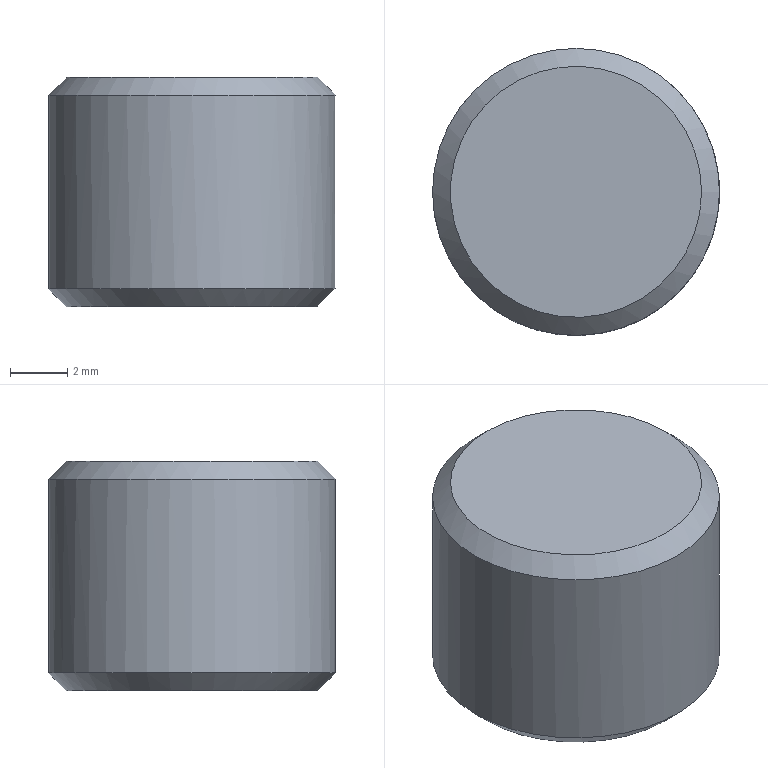Part | NX | features PG_666 2 | 1 solid | 5 faces | box 10.005 x 10.005 x 8 mm | volume 617.18 mm3 | plane 2 | cone 2 | cylinder 1 | commonest cylinder face diameters 10.005 x1
STEP:
#1=CARTESIAN_POINT('',(4307.859,-845.122,754.716));
#2=VERTEX_POINT('',#1);
#3=CARTESIAN_POINT('',(4312.236,-845.122,754.716));
#4=DIRECTION('',(0.,0.,-1.));
#5=DIRECTION('',(-1.,0.,0.));
#6=AXIS2_PLACEMENT_3D('',#3,#4,#5);
#7=CIRCLE('',#6,4.378);
#8=EDGE_CURVE('',#2,#2,#7,.T.);
#9=ORIENTED_EDGE('',*,*,#8,.T.);
#10=EDGE_LOOP('',(#9));
#11=FACE_BOUND('',#10,.T.);
#12=CARTESIAN_POINT('',(4312.236,-845.122,754.716));
#13=DIRECTION('',(0.,0.,-1.));
#14=DIRECTION('',(-1.,0.,0.));
#15=AXIS2_PLACEMENT_3D('',#12,#13,#14);
#16=PLANE('',#15);
#17=ADVANCED_FACE('',(#11),#16,.T.);
#18=CARTESIAN_POINT('',(4316.614,-845.122,762.716));
#19=VERTEX_POINT('',#18);
#20=CARTESIAN_POINT('',(4312.236,-845.122,762.716));
#21=DIRECTION('',(0.,0.,1.));
#22=DIRECTION('',(1.,0.,0.));
#23=AXIS2_PLACEMENT_3D('',#20,#21,#22);
#24=CIRCLE('',#23,4.378);
#25=EDGE_CURVE('',#19,#19,#24,.T.);
#26=ORIENTED_EDGE('',*,*,#25,.T.);
#27=EDGE_LOOP('',(#26));
#28=FACE_BOUND('',#27,.T.);
#29=CARTESIAN_POINT('',(4312.236,-845.122,762.716));
#30=DIRECTION('',(0.,0.,1.));
#31=DIRECTION('',(1.,0.,0.));
#32=AXIS2_PLACEMENT_3D('',#29,#30,#31);
#33=PLANE('',#32);
#34=ADVANCED_FACE('',(#28),#33,.T.);
#35=CARTESIAN_POINT('',(4317.239,-845.122,762.091));
#36=VERTEX_POINT('',#35);
#37=CARTESIAN_POINT('',(4312.236,-845.122,762.091));
#38=DIRECTION('',(0.,0.,1.));
#39=DIRECTION('',(1.,0.,0.));
#40=AXIS2_PLACEMENT_3D('',#37,#38,#39);
#41=CIRCLE('',#40,5.003);
#42=EDGE_CURVE('',#36,#36,#41,.F.);
#43=ORIENTED_EDGE('',*,*,#42,.T.);
#44=EDGE_LOOP('',(#43));
#45=FACE_BOUND('',#44,.T.);
#46=CARTESIAN_POINT('',(4307.234,-845.122,755.341));
#47=VERTEX_POINT('',#46);
#48=CARTESIAN_POINT('',(4312.236,-845.122,755.341));
#49=DIRECTION('',(0.,0.,-1.));
#50=DIRECTION('',(-1.,0.,0.));
#51=AXIS2_PLACEMENT_3D('',#48,#49,#50);
#52=CIRCLE('',#51,5.003);
#53=EDGE_CURVE('',#47,#47,#52,.F.);
#54=ORIENTED_EDGE('',*,*,#53,.T.);
#55=EDGE_LOOP('',(#54));
#56=FACE_BOUND('',#55,.T.);
#57=CARTESIAN_POINT('',(4312.236,-845.122,823.716));
#58=DIRECTION('',(0.,0.,-1.));
#59=DIRECTION('',(-1.,0.,0.));
#60=AXIS2_PLACEMENT_3D('',#57,#58,#59);
#61=CYLINDRICAL_SURFACE('',#60,5.003);
#62=ADVANCED_FACE('',(#45,#56),#61,.T.);
#63=ORIENTED_EDGE('',*,*,#25,.F.);
#64=EDGE_LOOP('',(#63));
#65=FACE_BOUND('',#64,.T.);
#66=ORIENTED_EDGE('',*,*,#42,.F.);
#67=EDGE_LOOP('',(#66));
#68=FACE_BOUND('',#67,.T.);
#69=CARTESIAN_POINT('',(4312.236,-845.122,762.091));
#70=DIRECTION('',(0.,0.,-1.));
#71=DIRECTION('',(-1.,0.,0.));
#72=AXIS2_PLACEMENT_3D('',#69,#70,#71);
#73=CONICAL_SURFACE('',#72,5.003,0.7854);
#74=ADVANCED_FACE('',(#65,#68),#73,.T.);
#75=ORIENTED_EDGE('',*,*,#8,.F.);
#76=EDGE_LOOP('',(#75));
#77=FACE_BOUND('',#76,.T.);
#78=ORIENTED_EDGE('',*,*,#53,.F.);
#79=EDGE_LOOP('',(#78));
#80=FACE_BOUND('',#79,.T.);
#81=CARTESIAN_POINT('',(4312.236,-845.122,755.341));
#82=DIRECTION('',(0.,0.,1.));
#83=DIRECTION('',(1.,0.,0.));
#84=AXIS2_PLACEMENT_3D('',#81,#82,#83);
#85=CONICAL_SURFACE('',#84,5.003,0.7854);
#86=ADVANCED_FACE('',(#77,#80),#85,.T.);
#87=CLOSED_SHELL('',(#17,#34,#62,#74,#86));
#88=MANIFOLD_SOLID_BREP('',#87);
#89=(LENGTH_UNIT()NAMED_UNIT(*)SI_UNIT(.MILLI.,.METRE.));
#90=UNCERTAINTY_MEASURE_WITH_UNIT(LENGTH_MEASURE(0.00001),#89,'','');
#91=(NAMED_UNIT(*)PLANE_ANGLE_UNIT()SI_UNIT($,.RADIAN.));
#92=(NAMED_UNIT(*)SI_UNIT($,.STERADIAN.)SOLID_ANGLE_UNIT());
#93=(GEOMETRIC_REPRESENTATION_CONTEXT(3)GLOBAL_UNCERTAINTY_ASSIGNED_CONTEXT((#90))GLOBAL_UNIT_ASSIGNED_CONTEXT((#89,#91,#92))REPRESENTATION_CONTEXT('',''));
#94=ADVANCED_BREP_SHAPE_REPRESENTATION('',(#88),#93);